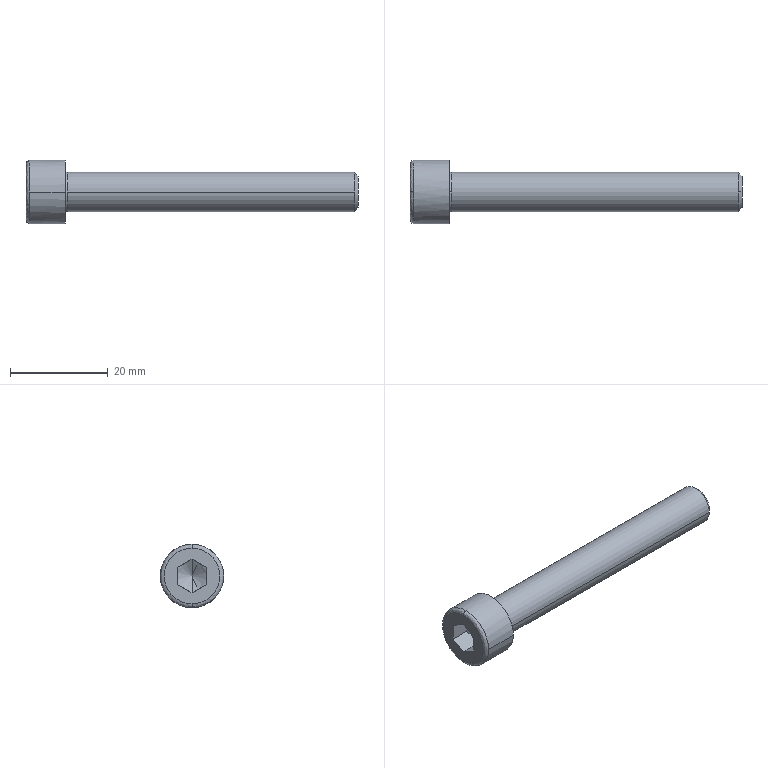Part | SolidWorks | features BaseBody 1 | 1 solid | 21 faces | box 68 x 13 x 13 mm | volume 3917 mm3 | plane 9 | spline 4 | cylinder 4 | cone 4 | commonest cylinder face diameters 8 x2 13 x2
STEP:
#1=CARTESIAN_POINT('',(0.,0.,4.4));
#2=VERTEX_POINT('',#1);
#3=CARTESIAN_POINT('',(0.,0.,-4.4));
#4=VERTEX_POINT('',#3);
#5=CARTESIAN_POINT('',(0.,0.,4.4));
#6=CARTESIAN_POINT('',(0.,0.2796,4.4));
#7=CARTESIAN_POINT('',(0.,0.6917,4.361));
#8=CARTESIAN_POINT('',(0.,1.16,4.249));
#9=CARTESIAN_POINT('',(0.,1.391,4.176));
#10=CARTESIAN_POINT('',(0.,1.489,4.141));
#11=CARTESIAN_POINT('',(0.,1.554,4.116));
#12=CARTESIAN_POINT('',(0.,1.585,4.105));
#13=CARTESIAN_POINT('',(0.,1.758,4.036));
#14=CARTESIAN_POINT('',(0.,1.96,3.944));
#15=CARTESIAN_POINT('',(0.,2.154,3.837));
#16=CARTESIAN_POINT('',(0.,2.282,3.763));
#17=CARTESIAN_POINT('',(0.,2.344,3.724));
#18=CARTESIAN_POINT('',(0.,2.662,3.517));
#19=CARTESIAN_POINT('',(0.,2.897,3.326));
#20=CARTESIAN_POINT('',(0.,3.219,3.004));
#21=CARTESIAN_POINT('',(0.,3.37,2.836));
#22=CARTESIAN_POINT('',(0.,3.509,2.656));
#23=CARTESIAN_POINT('',(0.,3.598,2.534));
#24=CARTESIAN_POINT('',(0.,3.642,2.47));
#25=CARTESIAN_POINT('',(0.,3.764,2.283));
#26=CARTESIAN_POINT('',(0.,3.876,2.092));
#27=CARTESIAN_POINT('',(0.,3.989,1.859));
#28=CARTESIAN_POINT('',(0.,4.034,1.757));
#29=CARTESIAN_POINT('',(0.,4.063,1.689));
#30=CARTESIAN_POINT('',(0.,4.078,1.652));
#31=CARTESIAN_POINT('',(0.,4.297,1.099));
#32=CARTESIAN_POINT('',(0.,4.4,0.5594));
#33=CARTESIAN_POINT('',(0.,4.4,-0.2797));
#34=CARTESIAN_POINT('',(0.,4.374,-0.5547));
#35=CARTESIAN_POINT('',(0.,4.297,-0.9596));
#36=CARTESIAN_POINT('',(0.,4.249,-1.16));
#37=CARTESIAN_POINT('',(0.,4.175,-1.391));
#38=CARTESIAN_POINT('',(0.,4.141,-1.489));
#39=CARTESIAN_POINT('',(0.,4.116,-1.555));
#40=CARTESIAN_POINT('',(0.,4.105,-1.585));
#41=CARTESIAN_POINT('',(0.,4.036,-1.758));
#42=CARTESIAN_POINT('',(0.,3.944,-1.96));
#43=CARTESIAN_POINT('',(0.,3.837,-2.154));
#44=CARTESIAN_POINT('',(0.,3.763,-2.282));
#45=CARTESIAN_POINT('',(0.,3.724,-2.344));
#46=CARTESIAN_POINT('',(0.,3.517,-2.662));
#47=CARTESIAN_POINT('',(0.,3.326,-2.897));
#48=CARTESIAN_POINT('',(0.,3.004,-3.219));
#49=CARTESIAN_POINT('',(0.,2.836,-3.37));
#50=CARTESIAN_POINT('',(0.,2.656,-3.509));
#51=CARTESIAN_POINT('',(0.,2.534,-3.598));
#52=CARTESIAN_POINT('',(0.,2.47,-3.642));
#53=CARTESIAN_POINT('',(0.,2.283,-3.764));
#54=CARTESIAN_POINT('',(0.,2.092,-3.876));
#55=CARTESIAN_POINT('',(0.,1.859,-3.989));
#56=CARTESIAN_POINT('',(0.,1.74,-4.042));
#57=CARTESIAN_POINT('',(0.,1.689,-4.063));
#58=CARTESIAN_POINT('',(0.,1.654,-4.077));
#59=CARTESIAN_POINT('',(0.,1.636,-4.085));
#60=CARTESIAN_POINT('',(0.,1.1,-4.297));
#61=CARTESIAN_POINT('',(0.,0.5592,-4.4));
#62=CARTESIAN_POINT('',(0.,0.,-4.4));
#63=B_SPLINE_CURVE_WITH_KNOTS('',3,(#5,#6,#7,#8,#9,#10,#11,#12,#13,#14,#15,#16,#17,#18,#19,#20,#21,#22,#23,#24,#25,#26,#27,#28,#29,#30,#31,#32,#33,#34,#35,#36,#37,#38,#39,#40,#41,#42,#43,#44,#45,#46,#47,#48,#49,#50,#51,#52,#53,#54,#55,#56,#57,#58,#59,#60,#61,#62),.UNSPECIFIED.,.F.,.F.,(4,1,1,1,2,2,1,2,2,2,1,2,2,1,1,2,2,2,2,1,1,2,2,1,2,2,2,1,2,2,1,1,1,2,2,4),(0.75,0.7812,0.7969,0.8047,0.8086,0.8125,0.8281,0.8359,0.8437,0.875,0.8906,0.8984,0.9062,0.9219,0.9297,0.9336,0.9375,1.,1.031,1.047,1.055,1.059,1.062,1.078,1.086,1.094,1.125,1.141,1.148,1.156,1.172,1.18,1.184,1.186,1.187,1.25),.UNSPECIFIED.);
#64=EDGE_CURVE('',#2,#4,#63,.T.);
#65=ORIENTED_EDGE('',*,*,#64,.F.);
#66=CARTESIAN_POINT('',(0.4,0.,4.));
#67=VERTEX_POINT('',#66);
#68=CARTESIAN_POINT('',(0.4,0.,4.4));
#69=DIRECTION('',(0.,-1.,0.));
#70=DIRECTION('',(0.,0.,1.));
#71=AXIS2_PLACEMENT_3D('',#68,#69,#70);
#72=CIRCLE('',#71,0.4);
#73=EDGE_CURVE('',#2,#67,#72,.T.);
#74=ORIENTED_EDGE('',*,*,#73,.T.);
#75=CARTESIAN_POINT('',(0.4,4.,0.));
#76=VERTEX_POINT('',#75);
#77=CARTESIAN_POINT('',(0.4,0.,0.));
#78=DIRECTION('',(1.,0.,0.));
#79=DIRECTION('',(0.,1.,0.));
#80=AXIS2_PLACEMENT_3D('',#77,#78,#79);
#81=CIRCLE('',#80,4.);
#82=EDGE_CURVE('',#76,#67,#81,.T.);
#83=ORIENTED_EDGE('',*,*,#82,.F.);
#84=CARTESIAN_POINT('',(0.4,0.,-4.));
#85=VERTEX_POINT('',#84);
#86=CARTESIAN_POINT('',(0.4,0.,0.));
#87=DIRECTION('',(1.,0.,0.));
#88=DIRECTION('',(0.,1.,0.));
#89=AXIS2_PLACEMENT_3D('',#86,#87,#88);
#90=CIRCLE('',#89,4.);
#91=EDGE_CURVE('',#85,#76,#90,.T.);
#92=ORIENTED_EDGE('',*,*,#91,.F.);
#93=CARTESIAN_POINT('',(0.4,0.,-4.4));
#94=DIRECTION('',(0.,1.,0.));
#95=DIRECTION('',(0.,0.,-1.));
#96=AXIS2_PLACEMENT_3D('',#93,#94,#95);
#97=CIRCLE('',#96,0.4);
#98=EDGE_CURVE('',#4,#85,#97,.T.);
#99=ORIENTED_EDGE('',*,*,#98,.F.);
#100=EDGE_LOOP('',(#65,#74,#83,#92,#99));
#101=FACE_OUTER_BOUND('',#100,.T.);
#102=CARTESIAN_POINT('',(0.,0.,-4.4));
#103=CARTESIAN_POINT('',(0.,8.8,-4.4));
#104=CARTESIAN_POINT('',(0.,8.8,4.4));
#105=CARTESIAN_POINT('',(0.,0.,4.4));
#106=CARTESIAN_POINT('',(0.,0.,-4.166));
#107=CARTESIAN_POINT('',(0.,8.331,-4.166));
#108=CARTESIAN_POINT('',(0.,8.331,4.166));
#109=CARTESIAN_POINT('',(0.,0.,4.166));
#110=CARTESIAN_POINT('',(0.1657,0.,-4.));
#111=CARTESIAN_POINT('',(0.1657,8.,-4.));
#112=CARTESIAN_POINT('',(0.1657,8.,4.));
#113=CARTESIAN_POINT('',(0.1657,0.,4.));
#114=CARTESIAN_POINT('',(0.4,0.,-4.));
#115=CARTESIAN_POINT('',(0.4,8.,-4.));
#116=CARTESIAN_POINT('',(0.4,8.,4.));
#117=CARTESIAN_POINT('',(0.4,0.,4.));
#118=(BOUNDED_SURFACE()B_SPLINE_SURFACE(3,3,((#102,#103,#104,#105),(#106,#107,#108,#109),(#110,#111,#112,#113),(#114,#115,#116,#117)),.UNSPECIFIED.,.F.,.F.,.F.)B_SPLINE_SURFACE_WITH_KNOTS((4,4),(4,4),(0.,1.),(0.,1.),.UNSPECIFIED.)GEOMETRIC_REPRESENTATION_ITEM()RATIONAL_B_SPLINE_SURFACE(((1.,0.3333,0.3333,1.),(0.8047,0.2682,0.2682,0.8047),(0.8047,0.2682,0.2682,0.8047),(1.,0.3333,0.3333,1.)))REPRESENTATION_ITEM('')SURFACE());
#119=ADVANCED_FACE('',(#101),#118,.F.);
#120=CARTESIAN_POINT('',(-7.2,0.,6.5));
#121=VERTEX_POINT('',#120);
#122=CARTESIAN_POINT('',(-7.2,-6.5,0.));
#123=VERTEX_POINT('',#122);
#124=CARTESIAN_POINT('',(-7.2,0.,0.));
#125=DIRECTION('',(1.,0.,0.));
#126=DIRECTION('',(0.,1.,0.));
#127=AXIS2_PLACEMENT_3D('',#124,#125,#126);
#128=CIRCLE('',#127,6.5);
#129=EDGE_CURVE('',#121,#123,#128,.T.);
#130=ORIENTED_EDGE('',*,*,#129,.F.);
#131=CARTESIAN_POINT('',(-8.,0.,5.7));
#132=VERTEX_POINT('',#131);
#133=CARTESIAN_POINT('',(-7.2,0.,5.7));
#134=DIRECTION('',(0.,-1.,0.));
#135=DIRECTION('',(0.,0.,1.));
#136=AXIS2_PLACEMENT_3D('',#133,#134,#135);
#137=CIRCLE('',#136,0.8);
#138=EDGE_CURVE('',#121,#132,#137,.T.);
#139=ORIENTED_EDGE('',*,*,#138,.T.);
#140=CARTESIAN_POINT('',(-8.,0.,-5.7));
#141=VERTEX_POINT('',#140);
#142=CARTESIAN_POINT('',(-8.,0.,5.7));
#143=CARTESIAN_POINT('',(-8.,-11.4,5.7));
#144=CARTESIAN_POINT('',(-8.,-11.4,-5.7));
#145=CARTESIAN_POINT('',(-8.,0.,-5.7));
#146=(BOUNDED_CURVE()B_SPLINE_CURVE(3,(#142,#143,#144,#145),.UNSPECIFIED.,.F.,.F.)B_SPLINE_CURVE_WITH_KNOTS((4,4),(0.25,0.75),.UNSPECIFIED.)CURVE()GEOMETRIC_REPRESENTATION_ITEM()RATIONAL_B_SPLINE_CURVE((1.,0.3333,0.3333,1.))REPRESENTATION_ITEM(''));
#147=EDGE_CURVE('',#132,#141,#146,.T.);
#148=ORIENTED_EDGE('',*,*,#147,.T.);
#149=CARTESIAN_POINT('',(-7.2,0.,-6.5));
#150=VERTEX_POINT('',#149);
#151=CARTESIAN_POINT('',(-7.2,0.,-5.7));
#152=DIRECTION('',(0.,1.,0.));
#153=DIRECTION('',(0.,0.,-1.));
#154=AXIS2_PLACEMENT_3D('',#151,#152,#153);
#155=CIRCLE('',#154,0.8);
#156=EDGE_CURVE('',#150,#141,#155,.T.);
#157=ORIENTED_EDGE('',*,*,#156,.F.);
#158=CARTESIAN_POINT('',(-7.2,0.,0.));
#159=DIRECTION('',(1.,0.,0.));
#160=DIRECTION('',(0.,1.,0.));
#161=AXIS2_PLACEMENT_3D('',#158,#159,#160);
#162=CIRCLE('',#161,6.5);
#163=EDGE_CURVE('',#123,#150,#162,.T.);
#164=ORIENTED_EDGE('',*,*,#163,.F.);
#165=EDGE_LOOP('',(#130,#139,#148,#157,#164));
#166=FACE_OUTER_BOUND('',#165,.T.);
#167=CARTESIAN_POINT('',(-7.2,0.,6.5));
#168=CARTESIAN_POINT('',(-7.2,-13.,6.5));
#169=CARTESIAN_POINT('',(-7.2,-13.,-6.5));
#170=CARTESIAN_POINT('',(-7.2,0.,-6.5));
#171=CARTESIAN_POINT('',(-7.669,0.,6.5));
#172=CARTESIAN_POINT('',(-7.669,-13.,6.5));
#173=CARTESIAN_POINT('',(-7.669,-13.,-6.5));
#174=CARTESIAN_POINT('',(-7.669,0.,-6.5));
#175=CARTESIAN_POINT('',(-8.,0.,6.169));
#176=CARTESIAN_POINT('',(-8.,-12.337,6.169));
#177=CARTESIAN_POINT('',(-8.,-12.337,-6.169));
#178=CARTESIAN_POINT('',(-8.,0.,-6.169));
#179=CARTESIAN_POINT('',(-8.,0.,5.7));
#180=CARTESIAN_POINT('',(-8.,-11.4,5.7));
#181=CARTESIAN_POINT('',(-8.,-11.4,-5.7));
#182=CARTESIAN_POINT('',(-8.,0.,-5.7));
#183=(BOUNDED_SURFACE()B_SPLINE_SURFACE(3,3,((#167,#168,#169,#170),(#171,#172,#173,#174),(#175,#176,#177,#178),(#179,#180,#181,#182)),.UNSPECIFIED.,.F.,.F.,.T.)B_SPLINE_SURFACE_WITH_KNOTS((4,4),(4,4),(0.,1.),(0.,1.),.UNSPECIFIED.)GEOMETRIC_REPRESENTATION_ITEM()RATIONAL_B_SPLINE_SURFACE(((1.,0.3333,0.3333,1.),(0.8047,0.2682,0.2682,0.8047),(0.8047,0.2682,0.2682,0.8047),(1.,0.3333,0.3333,1.)))REPRESENTATION_ITEM('')SURFACE());
#184=ADVANCED_FACE('',(#166),#183,.T.);
#185=ORIENTED_EDGE('',*,*,#82,.T.);
#186=CARTESIAN_POINT('',(0.4,-4.,0.));
#187=VERTEX_POINT('',#186);
#188=CARTESIAN_POINT('',(0.4,0.,0.));
#189=DIRECTION('',(1.,0.,0.));
#190=DIRECTION('',(0.,1.,0.));
#191=AXIS2_PLACEMENT_3D('',#188,#189,#190);
#192=CIRCLE('',#191,4.);
#193=EDGE_CURVE('',#67,#187,#192,.T.);
#194=ORIENTED_EDGE('',*,*,#193,.T.);
#195=CARTESIAN_POINT('',(59.233,-4.,0.));
#196=VERTEX_POINT('',#195);
#197=CARTESIAN_POINT('',(46.,-4.,0.));
#198=DIRECTION('',(1.,0.,0.));
#199=VECTOR('',#198,1000.);
#200=LINE('',#197,#199);
#201=EDGE_CURVE('',#187,#196,#200,.T.);
#202=ORIENTED_EDGE('',*,*,#201,.T.);
#203=CARTESIAN_POINT('',(59.233,0.,4.));
#204=VERTEX_POINT('',#203);
#205=CARTESIAN_POINT('',(59.233,0.,0.));
#206=DIRECTION('',(-1.,0.,0.));
#207=DIRECTION('',(0.,1.,0.));
#208=AXIS2_PLACEMENT_3D('',#205,#206,#207);
#209=CIRCLE('',#208,4.);
#210=EDGE_CURVE('',#196,#204,#209,.T.);
#211=ORIENTED_EDGE('',*,*,#210,.T.);
#212=CARTESIAN_POINT('',(59.233,4.,0.));
#213=VERTEX_POINT('',#212);
#214=CARTESIAN_POINT('',(59.233,0.,0.));
#215=DIRECTION('',(-1.,0.,0.));
#216=DIRECTION('',(0.,1.,0.));
#217=AXIS2_PLACEMENT_3D('',#214,#215,#216);
#218=CIRCLE('',#217,4.);
#219=EDGE_CURVE('',#204,#213,#218,.T.);
#220=ORIENTED_EDGE('',*,*,#219,.T.);
#221=CARTESIAN_POINT('',(46.,4.,0.));
#222=DIRECTION('',(1.,0.,0.));
#223=VECTOR('',#222,1000.);
#224=LINE('',#221,#223);
#225=EDGE_CURVE('',#76,#213,#224,.T.);
#226=ORIENTED_EDGE('',*,*,#225,.F.);
#227=EDGE_LOOP('',(#185,#194,#202,#211,#220,#226));
#228=FACE_OUTER_BOUND('',#227,.T.);
#229=CARTESIAN_POINT('',(46.,0.,0.));
#230=DIRECTION('',(1.,0.,0.));
#231=DIRECTION('',(0.,1.,0.));
#232=AXIS2_PLACEMENT_3D('',#229,#230,#231);
#233=CYLINDRICAL_SURFACE('',#232,4.);
#234=ADVANCED_FACE('',(#228),#233,.T.);
#235=CARTESIAN_POINT('',(60.,0.,3.233));
#236=VERTEX_POINT('',#235);
#237=CARTESIAN_POINT('',(60.,0.,-3.233));
#238=VERTEX_POINT('',#237);
#239=CARTESIAN_POINT('',(60.,0.,0.));
#240=DIRECTION('',(-1.,0.,0.));
#241=DIRECTION('',(0.,0.,1.));
#242=AXIS2_PLACEMENT_3D('',#239,#240,#241);
#243=CIRCLE('',#242,3.233);
#244=EDGE_CURVE('',#236,#238,#243,.T.);
#245=ORIENTED_EDGE('',*,*,#244,.T.);
#246=CARTESIAN_POINT('',(59.233,0.,-4.));
#247=VERTEX_POINT('',#246);
#248=CARTESIAN_POINT('',(59.233,0.,-4.));
#249=DIRECTION('',(-0.7071,0.,-0.7071));
#250=VECTOR('',#249,1000.);
#251=LINE('',#248,#250);
#252=EDGE_CURVE('',#238,#247,#251,.T.);
#253=ORIENTED_EDGE('',*,*,#252,.T.);
#254=CARTESIAN_POINT('',(59.233,0.,0.));
#255=DIRECTION('',(-1.,0.,0.));
#256=DIRECTION('',(0.,1.,0.));
#257=AXIS2_PLACEMENT_3D('',#254,#255,#256);
#258=CIRCLE('',#257,4.);
#259=EDGE_CURVE('',#213,#247,#258,.T.);
#260=ORIENTED_EDGE('',*,*,#259,.F.);
#261=ORIENTED_EDGE('',*,*,#219,.F.);
#262=CARTESIAN_POINT('',(59.233,0.,4.));
#263=DIRECTION('',(-0.7071,0.,0.7071));
#264=VECTOR('',#263,1000.);
#265=LINE('',#262,#264);
#266=EDGE_CURVE('',#236,#204,#265,.T.);
#267=ORIENTED_EDGE('',*,*,#266,.F.);
#268=EDGE_LOOP('',(#245,#253,#260,#261,#267));
#269=FACE_OUTER_BOUND('',#268,.T.);
#270=CARTESIAN_POINT('',(59.233,0.,0.));
#271=DIRECTION('',(-1.,0.,0.));
#272=DIRECTION('',(0.,0.,1.));
#273=AXIS2_PLACEMENT_3D('',#270,#271,#272);
#274=CONICAL_SURFACE('',#273,4.,0.7854);
#275=ADVANCED_FACE('',(#269),#274,.T.);
#276=CARTESIAN_POINT('',(-7.2,6.5,0.));
#277=VERTEX_POINT('',#276);
#278=CARTESIAN_POINT('',(-7.2,0.,0.));
#279=DIRECTION('',(1.,0.,0.));
#280=DIRECTION('',(0.,1.,0.));
#281=AXIS2_PLACEMENT_3D('',#278,#279,#280);
#282=CIRCLE('',#281,6.5);
#283=EDGE_CURVE('',#277,#121,#282,.T.);
#284=ORIENTED_EDGE('',*,*,#283,.T.);
#285=ORIENTED_EDGE('',*,*,#129,.T.);
#286=CARTESIAN_POINT('',(0.,-6.5,0.));
#287=VERTEX_POINT('',#286);
#288=CARTESIAN_POINT('',(-4.,-6.5,0.));
#289=DIRECTION('',(1.,0.,0.));
#290=VECTOR('',#289,1000.);
#291=LINE('',#288,#290);
#292=EDGE_CURVE('',#123,#287,#291,.T.);
#293=ORIENTED_EDGE('',*,*,#292,.T.);
#294=CARTESIAN_POINT('',(0.,6.5,0.));
#295=VERTEX_POINT('',#294);
#296=CARTESIAN_POINT('',(0.,0.,0.));
#297=DIRECTION('',(1.,0.,0.));
#298=DIRECTION('',(0.,1.,0.));
#299=AXIS2_PLACEMENT_3D('',#296,#297,#298);
#300=CIRCLE('',#299,6.5);
#301=EDGE_CURVE('',#295,#287,#300,.T.);
#302=ORIENTED_EDGE('',*,*,#301,.F.);
#303=CARTESIAN_POINT('',(-4.,6.5,0.));
#304=DIRECTION('',(1.,0.,0.));
#305=VECTOR('',#304,1000.);
#306=LINE('',#303,#305);
#307=EDGE_CURVE('',#277,#295,#306,.T.);
#308=ORIENTED_EDGE('',*,*,#307,.F.);
#309=EDGE_LOOP('',(#284,#285,#293,#302,#308));
#310=FACE_OUTER_BOUND('',#309,.T.);
#311=CARTESIAN_POINT('',(-4.,0.,0.));
#312=DIRECTION('',(1.,0.,0.));
#313=DIRECTION('',(0.,1.,0.));
#314=AXIS2_PLACEMENT_3D('',#311,#312,#313);
#315=CYLINDRICAL_SURFACE('',#314,6.5);
#316=ADVANCED_FACE('',(#310),#315,.T.);
#317=CARTESIAN_POINT('',(-2.,0.,0.));
#318=VERTEX_POINT('',#317);
#319=CARTESIAN_POINT('',(-4.,0.,3.464));
#320=VERTEX_POINT('',#319);
#321=CARTESIAN_POINT('',(-4.012,0.,3.485));
#322=DIRECTION('',(-0.5,0.,0.866));
#323=VECTOR('',#322,1000.);
#324=LINE('',#321,#323);
#325=EDGE_CURVE('',#318,#320,#324,.T.);
#326=ORIENTED_EDGE('',*,*,#325,.F.);
#327=CARTESIAN_POINT('',(-4.,0.,-3.464));
#328=VERTEX_POINT('',#327);
#329=CARTESIAN_POINT('',(-4.012,0.,-3.485));
#330=DIRECTION('',(-0.5,0.,-0.866));
#331=VECTOR('',#330,1000.);
#332=LINE('',#329,#331);
#333=EDGE_CURVE('',#318,#328,#332,.T.);
#334=ORIENTED_EDGE('',*,*,#333,.T.);
#335=CARTESIAN_POINT('',(-4.,-3.,-1.732));
#336=VERTEX_POINT('',#335);
#337=CARTESIAN_POINT('',(-4.,0.,-3.464));
#338=CARTESIAN_POINT('',(-3.837,-0.4898,-3.181));
#339=CARTESIAN_POINT('',(-3.732,-0.987,-2.894));
#340=CARTESIAN_POINT('',(-3.732,-1.752,-2.452));
#341=CARTESIAN_POINT('',(-3.757,-2.007,-2.305));
#342=CARTESIAN_POINT('',(-3.851,-2.507,-2.016));
#343=CARTESIAN_POINT('',(-3.918,-2.755,-1.874));
#344=CARTESIAN_POINT('',(-4.,-3.,-1.732));
#345=B_SPLINE_CURVE_WITH_KNOTS('',3,(#337,#338,#339,#340,#341,#342,#343,#344),.UNSPECIFIED.,.F.,.F.,(4,2,2,4),(0.,0.001749,0.002624,0.003499),.UNSPECIFIED.);
#346=EDGE_CURVE('',#328,#336,#345,.T.);
#347=ORIENTED_EDGE('',*,*,#346,.T.);
#348=CARTESIAN_POINT('',(-4.,-3.,1.732));
#349=VERTEX_POINT('',#348);
#350=CARTESIAN_POINT('',(-4.,-3.,-1.732));
#351=CARTESIAN_POINT('',(-3.837,-3.,-1.166));
#352=CARTESIAN_POINT('',(-3.732,-3.,-0.5923));
#353=CARTESIAN_POINT('',(-3.732,-3.,0.2912));
#354=CARTESIAN_POINT('',(-3.757,-3.,0.5854));
#355=CARTESIAN_POINT('',(-3.851,-3.,1.163));
#356=CARTESIAN_POINT('',(-3.918,-3.,1.449));
#357=CARTESIAN_POINT('',(-4.,-3.,1.732));
#358=B_SPLINE_CURVE_WITH_KNOTS('',3,(#350,#351,#352,#353,#354,#355,#356,#357),.UNSPECIFIED.,.F.,.F.,(4,2,2,4),(0.,0.001749,0.002624,0.003499),.UNSPECIFIED.);
#359=EDGE_CURVE('',#336,#349,#358,.T.);
#360=ORIENTED_EDGE('',*,*,#359,.T.);
#361=CARTESIAN_POINT('',(-4.,-3.,1.732));
#362=CARTESIAN_POINT('',(-3.837,-2.51,2.015));
#363=CARTESIAN_POINT('',(-3.732,-2.013,2.302));
#364=CARTESIAN_POINT('',(-3.732,-1.248,2.744));
#365=CARTESIAN_POINT('',(-3.757,-0.993,2.891));
#366=CARTESIAN_POINT('',(-3.851,-0.4925,3.18));
#367=CARTESIAN_POINT('',(-3.918,-0.2452,3.323));
#368=CARTESIAN_POINT('',(-4.,0.,3.464));
#369=B_SPLINE_CURVE_WITH_KNOTS('',3,(#361,#362,#363,#364,#365,#366,#367,#368),.UNSPECIFIED.,.F.,.F.,(4,2,2,4),(0.,0.001749,0.002624,0.003499),.UNSPECIFIED.);
#370=EDGE_CURVE('',#349,#320,#369,.T.);
#371=ORIENTED_EDGE('',*,*,#370,.T.);
#372=EDGE_LOOP('',(#326,#334,#347,#360,#371));
#373=FACE_OUTER_BOUND('',#372,.T.);
#374=CARTESIAN_POINT('',(-4.012,0.,0.));
#375=DIRECTION('',(-1.,0.,0.));
#376=DIRECTION('',(0.,0.,1.));
#377=AXIS2_PLACEMENT_3D('',#374,#375,#376);
#378=CONICAL_SURFACE('',#377,3.485,1.047);
#379=ADVANCED_FACE('',(#373),#378,.F.);
#380=ORIENTED_EDGE('',*,*,#201,.F.);
#381=CARTESIAN_POINT('',(0.4,0.,0.));
#382=DIRECTION('',(1.,0.,0.));
#383=DIRECTION('',(0.,1.,0.));
#384=AXIS2_PLACEMENT_3D('',#381,#382,#383);
#385=CIRCLE('',#384,4.);
#386=EDGE_CURVE('',#187,#85,#385,.T.);
#387=ORIENTED_EDGE('',*,*,#386,.T.);
#388=ORIENTED_EDGE('',*,*,#91,.T.);
#389=ORIENTED_EDGE('',*,*,#225,.T.);
#390=ORIENTED_EDGE('',*,*,#259,.T.);
#391=CARTESIAN_POINT('',(59.233,0.,0.));
#392=DIRECTION('',(-1.,0.,0.));
#393=DIRECTION('',(0.,1.,0.));
#394=AXIS2_PLACEMENT_3D('',#391,#392,#393);
#395=CIRCLE('',#394,4.);
#396=EDGE_CURVE('',#247,#196,#395,.T.);
#397=ORIENTED_EDGE('',*,*,#396,.T.);
#398=EDGE_LOOP('',(#380,#387,#388,#389,#390,#397));
#399=FACE_OUTER_BOUND('',#398,.T.);
#400=CARTESIAN_POINT('',(46.,0.,0.));
#401=DIRECTION('',(1.,0.,0.));
#402=DIRECTION('',(0.,1.,0.));
#403=AXIS2_PLACEMENT_3D('',#400,#401,#402);
#404=CYLINDRICAL_SURFACE('',#403,4.);
#405=ADVANCED_FACE('',(#399),#404,.T.);
#406=ORIENTED_EDGE('',*,*,#73,.F.);
#407=CARTESIAN_POINT('',(0.,0.,-4.4));
#408=CARTESIAN_POINT('',(0.,-0.2796,-4.4));
#409=CARTESIAN_POINT('',(0.,-0.6917,-4.361));
#410=CARTESIAN_POINT('',(0.,-1.16,-4.249));
#411=CARTESIAN_POINT('',(0.,-1.391,-4.176));
#412=CARTESIAN_POINT('',(0.,-1.489,-4.141));
#413=CARTESIAN_POINT('',(0.,-1.554,-4.116));
#414=CARTESIAN_POINT('',(0.,-1.585,-4.105));
#415=CARTESIAN_POINT('',(0.,-1.758,-4.036));
#416=CARTESIAN_POINT('',(0.,-1.96,-3.944));
#417=CARTESIAN_POINT('',(0.,-2.154,-3.837));
#418=CARTESIAN_POINT('',(0.,-2.282,-3.763));
#419=CARTESIAN_POINT('',(0.,-2.344,-3.724));
#420=CARTESIAN_POINT('',(0.,-2.662,-3.517));
#421=CARTESIAN_POINT('',(0.,-2.897,-3.326));
#422=CARTESIAN_POINT('',(0.,-3.219,-3.004));
#423=CARTESIAN_POINT('',(0.,-3.37,-2.836));
#424=CARTESIAN_POINT('',(0.,-3.509,-2.656));
#425=CARTESIAN_POINT('',(0.,-3.598,-2.534));
#426=CARTESIAN_POINT('',(0.,-3.642,-2.47));
#427=CARTESIAN_POINT('',(0.,-3.764,-2.283));
#428=CARTESIAN_POINT('',(0.,-3.876,-2.092));
#429=CARTESIAN_POINT('',(0.,-3.989,-1.859));
#430=CARTESIAN_POINT('',(0.,-4.042,-1.74));
#431=CARTESIAN_POINT('',(0.,-4.063,-1.689));
#432=CARTESIAN_POINT('',(0.,-4.077,-1.654));
#433=CARTESIAN_POINT('',(0.,-4.085,-1.636));
#434=CARTESIAN_POINT('',(0.,-4.297,-1.1));
#435=CARTESIAN_POINT('',(0.,-4.4,-0.5592));
#436=CARTESIAN_POINT('',(0.,-4.4,0.2796));
#437=CARTESIAN_POINT('',(0.,-4.361,0.6917));
#438=CARTESIAN_POINT('',(0.,-4.249,1.16));
#439=CARTESIAN_POINT('',(0.,-4.176,1.391));
#440=CARTESIAN_POINT('',(0.,-4.141,1.489));
#441=CARTESIAN_POINT('',(0.,-4.116,1.554));
#442=CARTESIAN_POINT('',(0.,-4.105,1.585));
#443=CARTESIAN_POINT('',(0.,-4.036,1.758));
#444=CARTESIAN_POINT('',(0.,-3.944,1.96));
#445=CARTESIAN_POINT('',(0.,-3.837,2.154));
#446=CARTESIAN_POINT('',(0.,-3.763,2.282));
#447=CARTESIAN_POINT('',(0.,-3.724,2.344));
#448=CARTESIAN_POINT('',(0.,-3.517,2.662));
#449=CARTESIAN_POINT('',(0.,-3.326,2.897));
#450=CARTESIAN_POINT('',(0.,-3.004,3.219));
#451=CARTESIAN_POINT('',(0.,-2.836,3.37));
#452=CARTESIAN_POINT('',(0.,-2.656,3.509));
#453=CARTESIAN_POINT('',(0.,-2.534,3.598));
#454=CARTESIAN_POINT('',(0.,-2.47,3.642));
#455=CARTESIAN_POINT('',(0.,-2.283,3.764));
#456=CARTESIAN_POINT('',(0.,-2.092,3.876));
#457=CARTESIAN_POINT('',(0.,-1.859,3.989));
#458=CARTESIAN_POINT('',(0.,-1.74,4.042));
#459=CARTESIAN_POINT('',(0.,-1.689,4.063));
#460=CARTESIAN_POINT('',(0.,-1.654,4.077));
#461=CARTESIAN_POINT('',(0.,-1.636,4.085));
#462=CARTESIAN_POINT('',(0.,-1.1,4.297));
#463=CARTESIAN_POINT('',(0.,-0.5592,4.4));
#464=CARTESIAN_POINT('',(0.,0.,4.4));
#465=B_SPLINE_CURVE_WITH_KNOTS('',3,(#407,#408,#409,#410,#411,#412,#413,#414,#415,#416,#417,#418,#419,#420,#421,#422,#423,#424,#425,#426,#427,#428,#429,#430,#431,#432,#433,#434,#435,#436,#437,#438,#439,#440,#441,#442,#443,#444,#445,#446,#447,#448,#449,#450,#451,#452,#453,#454,#455,#456,#457,#458,#459,#460,#461,#462,#463,#464),.UNSPECIFIED.,.F.,.F.,(4,1,1,1,2,2,1,2,2,2,1,2,2,1,1,1,2,2,2,1,1,1,2,2,1,2,2,2,1,2,2,1,1,1,2,2,4),(0.25,0.2812,0.2969,0.3047,0.3086,0.3125,0.3281,0.3359,0.3437,0.375,0.3906,0.3984,0.4062,0.4219,0.4297,0.4336,0.4355,0.4375,0.5,0.5312,0.5469,0.5547,0.5586,0.5625,0.5781,0.5859,0.5937,0.625,0.6406,0.6484,0.6562,0.6719,0.6797,0.6836,0.6855,0.6875,0.75),.UNSPECIFIED.);
#466=EDGE_CURVE('',#4,#2,#465,.T.);
#467=ORIENTED_EDGE('',*,*,#466,.F.);
#468=ORIENTED_EDGE('',*,*,#98,.T.);
#469=ORIENTED_EDGE('',*,*,#386,.F.);
#470=ORIENTED_EDGE('',*,*,#193,.F.);
#471=EDGE_LOOP('',(#406,#467,#468,#469,#470));
#472=FACE_OUTER_BOUND('',#471,.T.);
#473=CARTESIAN_POINT('',(0.,0.,4.4));
#474=CARTESIAN_POINT('',(0.,-8.8,4.4));
#475=CARTESIAN_POINT('',(0.,-8.8,-4.4));
#476=CARTESIAN_POINT('',(0.,0.,-4.4));
#477=CARTESIAN_POINT('',(0.,0.,4.166));
#478=CARTESIAN_POINT('',(0.,-8.331,4.166));
#479=CARTESIAN_POINT('',(0.,-8.331,-4.166));
#480=CARTESIAN_POINT('',(0.,0.,-4.166));
#481=CARTESIAN_POINT('',(0.1657,0.,4.));
#482=CARTESIAN_POINT('',(0.1657,-8.,4.));
#483=CARTESIAN_POINT('',(0.1657,-8.,-4.));
#484=CARTESIAN_POINT('',(0.1657,0.,-4.));
#485=CARTESIAN_POINT('',(0.4,0.,4.));
#486=CARTESIAN_POINT('',(0.4,-8.,4.));
#487=CARTESIAN_POINT('',(0.4,-8.,-4.));
#488=CARTESIAN_POINT('',(0.4,0.,-4.));
#489=(BOUNDED_SURFACE()B_SPLINE_SURFACE(3,3,((#473,#474,#475,#476),(#477,#478,#479,#480),(#481,#482,#483,#484),(#485,#486,#487,#488)),.UNSPECIFIED.,.F.,.F.,.F.)B_SPLINE_SURFACE_WITH_KNOTS((4,4),(4,4),(0.,1.),(0.,1.),.UNSPECIFIED.)GEOMETRIC_REPRESENTATION_ITEM()RATIONAL_B_SPLINE_SURFACE(((1.,0.3333,0.3333,1.),(0.8047,0.2682,0.2682,0.8047),(0.8047,0.2682,0.2682,0.8047),(1.,0.3333,0.3333,1.)))REPRESENTATION_ITEM('')SURFACE());
#490=ADVANCED_FACE('',(#472),#489,.F.);
#491=ORIENTED_EDGE('',*,*,#252,.F.);
#492=CARTESIAN_POINT('',(60.,0.,0.));
#493=DIRECTION('',(-1.,0.,0.));
#494=DIRECTION('',(0.,0.,1.));
#495=AXIS2_PLACEMENT_3D('',#492,#493,#494);
#496=CIRCLE('',#495,3.233);
#497=EDGE_CURVE('',#238,#236,#496,.T.);
#498=ORIENTED_EDGE('',*,*,#497,.T.);
#499=ORIENTED_EDGE('',*,*,#266,.T.);
#500=ORIENTED_EDGE('',*,*,#210,.F.);
#501=ORIENTED_EDGE('',*,*,#396,.F.);
#502=EDGE_LOOP('',(#491,#498,#499,#500,#501));
#503=FACE_OUTER_BOUND('',#502,.T.);
#504=CARTESIAN_POINT('',(59.233,0.,0.));
#505=DIRECTION('',(-1.,0.,0.));
#506=DIRECTION('',(0.,0.,1.));
#507=AXIS2_PLACEMENT_3D('',#504,#505,#506);
#508=CONICAL_SURFACE('',#507,4.,0.7854);
#509=ADVANCED_FACE('',(#503),#508,.T.);
#510=ORIENTED_EDGE('',*,*,#466,.T.);
#511=ORIENTED_EDGE('',*,*,#64,.T.);
#512=EDGE_LOOP('',(#510,#511));
#513=FACE_BOUND('',#512,.T.);
#514=ORIENTED_EDGE('',*,*,#301,.T.);
#515=CARTESIAN_POINT('',(0.,0.,0.));
#516=DIRECTION('',(1.,0.,0.));
#517=DIRECTION('',(0.,1.,0.));
#518=AXIS2_PLACEMENT_3D('',#515,#516,#517);
#519=CIRCLE('',#518,6.5);
#520=EDGE_CURVE('',#287,#295,#519,.T.);
#521=ORIENTED_EDGE('',*,*,#520,.T.);
#522=EDGE_LOOP('',(#514,#521));
#523=FACE_OUTER_BOUND('',#522,.T.);
#524=CARTESIAN_POINT('',(0.,5.25,0.));
#525=DIRECTION('',(1.,0.,0.));
#526=DIRECTION('',(0.,0.,-1.));
#527=AXIS2_PLACEMENT_3D('',#524,#525,#526);
#528=PLANE('',#527);
#529=ADVANCED_FACE('',(#513,#523),#528,.T.);
#530=ORIENTED_EDGE('',*,*,#244,.F.);
#531=ORIENTED_EDGE('',*,*,#497,.F.);
#532=EDGE_LOOP('',(#530,#531));
#533=FACE_OUTER_BOUND('',#532,.T.);
#534=CARTESIAN_POINT('',(60.,2.,0.));
#535=DIRECTION('',(1.,0.,0.));
#536=DIRECTION('',(0.,0.,-1.));
#537=AXIS2_PLACEMENT_3D('',#534,#535,#536);
#538=PLANE('',#537);
#539=ADVANCED_FACE('',(#533),#538,.T.);
#540=ORIENTED_EDGE('',*,*,#292,.F.);
#541=ORIENTED_EDGE('',*,*,#163,.T.);
#542=CARTESIAN_POINT('',(-7.2,0.,0.));
#543=DIRECTION('',(1.,0.,0.));
#544=DIRECTION('',(0.,1.,0.));
#545=AXIS2_PLACEMENT_3D('',#542,#543,#544);
#546=CIRCLE('',#545,6.5);
#547=EDGE_CURVE('',#150,#277,#546,.T.);
#548=ORIENTED_EDGE('',*,*,#547,.T.);
#549=ORIENTED_EDGE('',*,*,#307,.T.);
#550=ORIENTED_EDGE('',*,*,#520,.F.);
#551=EDGE_LOOP('',(#540,#541,#548,#549,#550));
#552=FACE_OUTER_BOUND('',#551,.T.);
#553=CARTESIAN_POINT('',(-4.,0.,0.));
#554=DIRECTION('',(1.,0.,0.));
#555=DIRECTION('',(0.,1.,0.));
#556=AXIS2_PLACEMENT_3D('',#553,#554,#555);
#557=CYLINDRICAL_SURFACE('',#556,6.5);
#558=ADVANCED_FACE('',(#552),#557,.T.);
#559=ORIENTED_EDGE('',*,*,#138,.F.);
#560=ORIENTED_EDGE('',*,*,#283,.F.);
#561=ORIENTED_EDGE('',*,*,#547,.F.);
#562=ORIENTED_EDGE('',*,*,#156,.T.);
#563=CARTESIAN_POINT('',(-8.,0.,-5.7));
#564=CARTESIAN_POINT('',(-8.,11.4,-5.7));
#565=CARTESIAN_POINT('',(-8.,11.4,5.7));
#566=CARTESIAN_POINT('',(-8.,0.,5.7));
#567=(BOUNDED_CURVE()B_SPLINE_CURVE(3,(#563,#564,#565,#566),.UNSPECIFIED.,.F.,.F.)B_SPLINE_CURVE_WITH_KNOTS((4,4),(0.75,1.25),.UNSPECIFIED.)CURVE()GEOMETRIC_REPRESENTATION_ITEM()RATIONAL_B_SPLINE_CURVE((1.,0.3333,0.3333,1.))REPRESENTATION_ITEM(''));
#568=EDGE_CURVE('',#141,#132,#567,.T.);
#569=ORIENTED_EDGE('',*,*,#568,.T.);
#570=EDGE_LOOP('',(#559,#560,#561,#562,#569));
#571=FACE_OUTER_BOUND('',#570,.T.);
#572=CARTESIAN_POINT('',(-7.2,0.,-6.5));
#573=CARTESIAN_POINT('',(-7.2,13.,-6.5));
#574=CARTESIAN_POINT('',(-7.2,13.,6.5));
#575=CARTESIAN_POINT('',(-7.2,0.,6.5));
#576=CARTESIAN_POINT('',(-7.669,0.,-6.5));
#577=CARTESIAN_POINT('',(-7.669,13.,-6.5));
#578=CARTESIAN_POINT('',(-7.669,13.,6.5));
#579=CARTESIAN_POINT('',(-7.669,0.,6.5));
#580=CARTESIAN_POINT('',(-8.,0.,-6.169));
#581=CARTESIAN_POINT('',(-8.,12.337,-6.169));
#582=CARTESIAN_POINT('',(-8.,12.337,6.169));
#583=CARTESIAN_POINT('',(-8.,0.,6.169));
#584=CARTESIAN_POINT('',(-8.,0.,-5.7));
#585=CARTESIAN_POINT('',(-8.,11.4,-5.7));
#586=CARTESIAN_POINT('',(-8.,11.4,5.7));
#587=CARTESIAN_POINT('',(-8.,0.,5.7));
#588=(BOUNDED_SURFACE()B_SPLINE_SURFACE(3,3,((#572,#573,#574,#575),(#576,#577,#578,#579),(#580,#581,#582,#583),(#584,#585,#586,#587)),.UNSPECIFIED.,.F.,.F.,.F.)B_SPLINE_SURFACE_WITH_KNOTS((4,4),(4,4),(0.,1.),(0.,1.),.UNSPECIFIED.)GEOMETRIC_REPRESENTATION_ITEM()RATIONAL_B_SPLINE_SURFACE(((1.,0.3333,0.3333,1.),(0.8047,0.2682,0.2682,0.8047),(0.8047,0.2682,0.2682,0.8047),(1.,0.3333,0.3333,1.)))REPRESENTATION_ITEM('')SURFACE());
#589=ADVANCED_FACE('',(#571),#588,.T.);
#590=CARTESIAN_POINT('',(-8.,-3.,-1.732));
#591=VERTEX_POINT('',#590);
#592=CARTESIAN_POINT('',(-8.,0.,-3.464));
#593=VERTEX_POINT('',#592);
#594=CARTESIAN_POINT('',(-8.,-3.,-1.732));
#595=DIRECTION('',(0.,0.866,-0.5));
#596=VECTOR('',#595,1000.);
#597=LINE('',#594,#596);
#598=EDGE_CURVE('',#591,#593,#597,.T.);
#599=ORIENTED_EDGE('',*,*,#598,.T.);
#600=CARTESIAN_POINT('',(-8.,3.,-1.732));
#601=VERTEX_POINT('',#600);
#602=CARTESIAN_POINT('',(-8.,0.,-3.464));
#603=DIRECTION('',(0.,0.866,0.5));
#604=VECTOR('',#603,1000.);
#605=LINE('',#602,#604);
#606=EDGE_CURVE('',#593,#601,#605,.T.);
#607=ORIENTED_EDGE('',*,*,#606,.T.);
#608=CARTESIAN_POINT('',(-8.,3.,1.732));
#609=VERTEX_POINT('',#608);
#610=CARTESIAN_POINT('',(-8.,3.,0.));
#611=DIRECTION('',(0.,0.,1.));
#612=VECTOR('',#611,1000.);
#613=LINE('',#610,#612);
#614=EDGE_CURVE('',#601,#609,#613,.T.);
#615=ORIENTED_EDGE('',*,*,#614,.T.);
#616=CARTESIAN_POINT('',(-8.,0.,3.464));
#617=VERTEX_POINT('',#616);
#618=CARTESIAN_POINT('',(-8.,3.,1.732));
#619=DIRECTION('',(0.,-0.866,0.5));
#620=VECTOR('',#619,1000.);
#621=LINE('',#618,#620);
#622=EDGE_CURVE('',#609,#617,#621,.T.);
#623=ORIENTED_EDGE('',*,*,#622,.T.);
#624=CARTESIAN_POINT('',(-8.,-3.,1.732));
#625=VERTEX_POINT('',#624);
#626=CARTESIAN_POINT('',(-8.,0.,3.464));
#627=DIRECTION('',(0.,-0.866,-0.5));
#628=VECTOR('',#627,1000.);
#629=LINE('',#626,#628);
#630=EDGE_CURVE('',#617,#625,#629,.T.);
#631=ORIENTED_EDGE('',*,*,#630,.T.);
#632=CARTESIAN_POINT('',(-8.,-3.,0.));
#633=DIRECTION('',(0.,0.,-1.));
#634=VECTOR('',#633,1000.);
#635=LINE('',#632,#634);
#636=EDGE_CURVE('',#625,#591,#635,.T.);
#637=ORIENTED_EDGE('',*,*,#636,.T.);
#638=EDGE_LOOP('',(#599,#607,#615,#623,#631,#637));
#639=FACE_BOUND('',#638,.T.);
#640=ORIENTED_EDGE('',*,*,#568,.F.);
#641=ORIENTED_EDGE('',*,*,#147,.F.);
#642=EDGE_LOOP('',(#640,#641));
#643=FACE_OUTER_BOUND('',#642,.T.);
#644=CARTESIAN_POINT('',(-8.,4.982,0.));
#645=DIRECTION('',(-1.,0.,0.));
#646=DIRECTION('',(0.,0.,1.));
#647=AXIS2_PLACEMENT_3D('',#644,#645,#646);
#648=PLANE('',#647);
#649=ADVANCED_FACE('',(#639,#643),#648,.T.);
#650=CARTESIAN_POINT('',(-4.,3.,-1.732));
#651=VERTEX_POINT('',#650);
#652=CARTESIAN_POINT('',(-8.,3.,-1.732));
#653=DIRECTION('',(1.,0.,0.));
#654=VECTOR('',#653,1000.);
#655=LINE('',#652,#654);
#656=EDGE_CURVE('',#601,#651,#655,.T.);
#657=ORIENTED_EDGE('',*,*,#656,.F.);
#658=ORIENTED_EDGE('',*,*,#606,.F.);
#659=CARTESIAN_POINT('',(-8.,0.,-3.464));
#660=DIRECTION('',(-1.,0.,0.));
#661=VECTOR('',#660,1000.);
#662=LINE('',#659,#661);
#663=EDGE_CURVE('',#328,#593,#662,.T.);
#664=ORIENTED_EDGE('',*,*,#663,.F.);
#665=CARTESIAN_POINT('',(-4.,3.,-1.732));
#666=CARTESIAN_POINT('',(-3.837,2.51,-2.015));
#667=CARTESIAN_POINT('',(-3.732,2.013,-2.302));
#668=CARTESIAN_POINT('',(-3.732,1.248,-2.744));
#669=CARTESIAN_POINT('',(-3.757,0.993,-2.891));
#670=CARTESIAN_POINT('',(-3.851,0.4925,-3.18));
#671=CARTESIAN_POINT('',(-3.918,0.2452,-3.323));
#672=CARTESIAN_POINT('',(-4.,0.,-3.464));
#673=B_SPLINE_CURVE_WITH_KNOTS('',3,(#665,#666,#667,#668,#669,#670,#671,#672),.UNSPECIFIED.,.F.,.F.,(4,2,2,4),(0.,0.001749,0.002624,0.003499),.UNSPECIFIED.);
#674=EDGE_CURVE('',#651,#328,#673,.T.);
#675=ORIENTED_EDGE('',*,*,#674,.F.);
#676=EDGE_LOOP('',(#657,#658,#664,#675));
#677=FACE_OUTER_BOUND('',#676,.T.);
#678=CARTESIAN_POINT('',(-8.,3.,-1.732));
#679=DIRECTION('',(0.,0.5,-0.866));
#680=DIRECTION('',(0.,0.866,0.5));
#681=AXIS2_PLACEMENT_3D('',#678,#679,#680);
#682=PLANE('',#681);
#683=ADVANCED_FACE('',(#677),#682,.F.);
#684=ORIENTED_EDGE('',*,*,#663,.T.);
#685=ORIENTED_EDGE('',*,*,#598,.F.);
#686=CARTESIAN_POINT('',(-8.,-3.,-1.732));
#687=DIRECTION('',(-1.,0.,0.));
#688=VECTOR('',#687,1000.);
#689=LINE('',#686,#688);
#690=EDGE_CURVE('',#336,#591,#689,.T.);
#691=ORIENTED_EDGE('',*,*,#690,.F.);
#692=ORIENTED_EDGE('',*,*,#346,.F.);
#693=EDGE_LOOP('',(#684,#685,#691,#692));
#694=FACE_OUTER_BOUND('',#693,.T.);
#695=CARTESIAN_POINT('',(-8.,0.,-3.464));
#696=DIRECTION('',(0.,-0.5,-0.866));
#697=DIRECTION('',(0.,0.866,-0.5));
#698=AXIS2_PLACEMENT_3D('',#695,#696,#697);
#699=PLANE('',#698);
#700=ADVANCED_FACE('',(#694),#699,.F.);
#701=ORIENTED_EDGE('',*,*,#690,.T.);
#702=ORIENTED_EDGE('',*,*,#636,.F.);
#703=CARTESIAN_POINT('',(-8.,-3.,1.732));
#704=DIRECTION('',(-1.,0.,0.));
#705=VECTOR('',#704,1000.);
#706=LINE('',#703,#705);
#707=EDGE_CURVE('',#349,#625,#706,.T.);
#708=ORIENTED_EDGE('',*,*,#707,.F.);
#709=ORIENTED_EDGE('',*,*,#359,.F.);
#710=EDGE_LOOP('',(#701,#702,#708,#709));
#711=FACE_OUTER_BOUND('',#710,.T.);
#712=CARTESIAN_POINT('',(-8.,-3.,-1.732));
#713=DIRECTION('',(0.,-1.,0.));
#714=DIRECTION('',(0.,0.,-1.));
#715=AXIS2_PLACEMENT_3D('',#712,#713,#714);
#716=PLANE('',#715);
#717=ADVANCED_FACE('',(#711),#716,.F.);
#718=ORIENTED_EDGE('',*,*,#707,.T.);
#719=ORIENTED_EDGE('',*,*,#630,.F.);
#720=CARTESIAN_POINT('',(-8.,0.,3.464));
#721=DIRECTION('',(-1.,0.,0.));
#722=VECTOR('',#721,1000.);
#723=LINE('',#720,#722);
#724=EDGE_CURVE('',#320,#617,#723,.T.);
#725=ORIENTED_EDGE('',*,*,#724,.F.);
#726=ORIENTED_EDGE('',*,*,#370,.F.);
#727=EDGE_LOOP('',(#718,#719,#725,#726));
#728=FACE_OUTER_BOUND('',#727,.T.);
#729=CARTESIAN_POINT('',(-8.,-3.,1.732));
#730=DIRECTION('',(0.,-0.5,0.866));
#731=DIRECTION('',(0.,-0.866,-0.5));
#732=AXIS2_PLACEMENT_3D('',#729,#730,#731);
#733=PLANE('',#732);
#734=ADVANCED_FACE('',(#728),#733,.F.);
#735=ORIENTED_EDGE('',*,*,#724,.T.);
#736=ORIENTED_EDGE('',*,*,#622,.F.);
#737=CARTESIAN_POINT('',(-4.,3.,1.732));
#738=VERTEX_POINT('',#737);
#739=CARTESIAN_POINT('',(-8.,3.,1.732));
#740=DIRECTION('',(-1.,0.,0.));
#741=VECTOR('',#740,1000.);
#742=LINE('',#739,#741);
#743=EDGE_CURVE('',#738,#609,#742,.T.);
#744=ORIENTED_EDGE('',*,*,#743,.F.);
#745=CARTESIAN_POINT('',(-4.,0.,3.464));
#746=CARTESIAN_POINT('',(-3.837,0.4898,3.181));
#747=CARTESIAN_POINT('',(-3.732,0.987,2.894));
#748=CARTESIAN_POINT('',(-3.732,1.752,2.452));
#749=CARTESIAN_POINT('',(-3.757,2.007,2.305));
#750=CARTESIAN_POINT('',(-3.851,2.507,2.016));
#751=CARTESIAN_POINT('',(-3.918,2.755,1.874));
#752=CARTESIAN_POINT('',(-4.,3.,1.732));
#753=B_SPLINE_CURVE_WITH_KNOTS('',3,(#745,#746,#747,#748,#749,#750,#751,#752),.UNSPECIFIED.,.F.,.F.,(4,2,2,4),(0.,0.001749,0.002624,0.003499),.UNSPECIFIED.);
#754=EDGE_CURVE('',#320,#738,#753,.T.);
#755=ORIENTED_EDGE('',*,*,#754,.F.);
#756=EDGE_LOOP('',(#735,#736,#744,#755));
#757=FACE_OUTER_BOUND('',#756,.T.);
#758=CARTESIAN_POINT('',(-8.,0.,3.464));
#759=DIRECTION('',(0.,0.5,0.866));
#760=DIRECTION('',(0.,-0.866,0.5));
#761=AXIS2_PLACEMENT_3D('',#758,#759,#760);
#762=PLANE('',#761);
#763=ADVANCED_FACE('',(#757),#762,.F.);
#764=ORIENTED_EDGE('',*,*,#743,.T.);
#765=ORIENTED_EDGE('',*,*,#614,.F.);
#766=ORIENTED_EDGE('',*,*,#656,.T.);
#767=CARTESIAN_POINT('',(-4.,3.,1.732));
#768=CARTESIAN_POINT('',(-3.837,3.,1.166));
#769=CARTESIAN_POINT('',(-3.732,3.,0.5923));
#770=CARTESIAN_POINT('',(-3.732,3.,-0.2912));
#771=CARTESIAN_POINT('',(-3.757,3.,-0.5854));
#772=CARTESIAN_POINT('',(-3.851,3.,-1.163));
#773=CARTESIAN_POINT('',(-3.918,3.,-1.449));
#774=CARTESIAN_POINT('',(-4.,3.,-1.732));
#775=B_SPLINE_CURVE_WITH_KNOTS('',3,(#767,#768,#769,#770,#771,#772,#773,#774),.UNSPECIFIED.,.F.,.F.,(4,2,2,4),(0.,0.001749,0.002624,0.003499),.UNSPECIFIED.);
#776=EDGE_CURVE('',#738,#651,#775,.T.);
#777=ORIENTED_EDGE('',*,*,#776,.F.);
#778=EDGE_LOOP('',(#764,#765,#766,#777));
#779=FACE_OUTER_BOUND('',#778,.T.);
#780=CARTESIAN_POINT('',(-8.,3.,1.732));
#781=DIRECTION('',(0.,1.,0.));
#782=DIRECTION('',(0.,0.,1.));
#783=AXIS2_PLACEMENT_3D('',#780,#781,#782);
#784=PLANE('',#783);
#785=ADVANCED_FACE('',(#779),#784,.F.);
#786=ORIENTED_EDGE('',*,*,#333,.F.);
#787=ORIENTED_EDGE('',*,*,#325,.T.);
#788=ORIENTED_EDGE('',*,*,#754,.T.);
#789=ORIENTED_EDGE('',*,*,#776,.T.);
#790=ORIENTED_EDGE('',*,*,#674,.T.);
#791=EDGE_LOOP('',(#786,#787,#788,#789,#790));
#792=FACE_OUTER_BOUND('',#791,.T.);
#793=CARTESIAN_POINT('',(-4.012,0.,0.));
#794=DIRECTION('',(-1.,0.,0.));
#795=DIRECTION('',(0.,0.,1.));
#796=AXIS2_PLACEMENT_3D('',#793,#794,#795);
#797=CONICAL_SURFACE('',#796,3.485,1.047);
#798=ADVANCED_FACE('',(#792),#797,.F.);
#799=CLOSED_SHELL('',(#119,#184,#234,#275,#316,#379,#405,#490,#509,#529,#539,#558,#589,#649,#683,#700,#717,#734,#763,#785,#798));
#800=MANIFOLD_SOLID_BREP('',#799);
#801=CARTESIAN_POINT('',(0.,0.,0.));
#802=DIRECTION('',(0.,0.,1.));
#803=DIRECTION('',(1.,0.,0.));
#804=AXIS2_PLACEMENT_3D('',#801,#802,#803);
#805=(LENGTH_UNIT()NAMED_UNIT(*)SI_UNIT(.MILLI.,.METRE.));
#806=UNCERTAINTY_MEASURE_WITH_UNIT(LENGTH_MEASURE(0.00001),#805,'','');
#807=(NAMED_UNIT(*)PLANE_ANGLE_UNIT()SI_UNIT($,.RADIAN.));
#808=(NAMED_UNIT(*)SI_UNIT($,.STERADIAN.)SOLID_ANGLE_UNIT());
#809=(GEOMETRIC_REPRESENTATION_CONTEXT(3)GLOBAL_UNCERTAINTY_ASSIGNED_CONTEXT((#806))GLOBAL_UNIT_ASSIGNED_CONTEXT((#805,#807,#808))REPRESENTATION_CONTEXT('',''));
#810=ADVANCED_BREP_SHAPE_REPRESENTATION('',(#800,#804),#809);